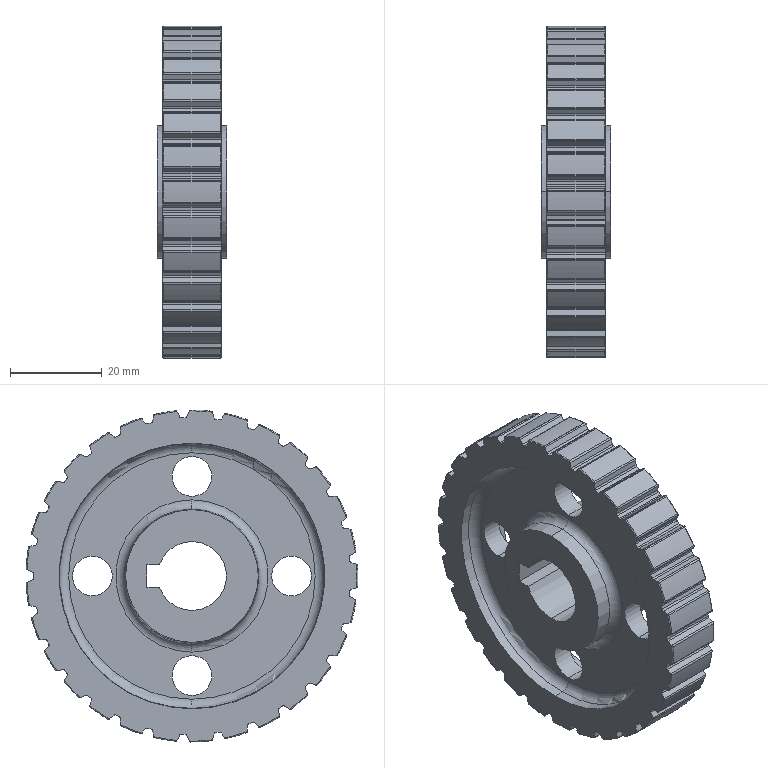Part | SolidWorks | features Cut 3, CirPattern 2, ICE 2, Chamfer 1, Fillet 1, RefAxis 1, Revolution 1 | 1 solid | 349 faces | box 15.24 x 72.254 x 72.292 mm | volume 33206 mm3 | cylinder 206 | torus 68 | plane 67 | cone 8 | commonest cylinder face diameters 0.76 x68 0.82 x68 72.292 x30 68.992 x29 8.675 x8 15 x3